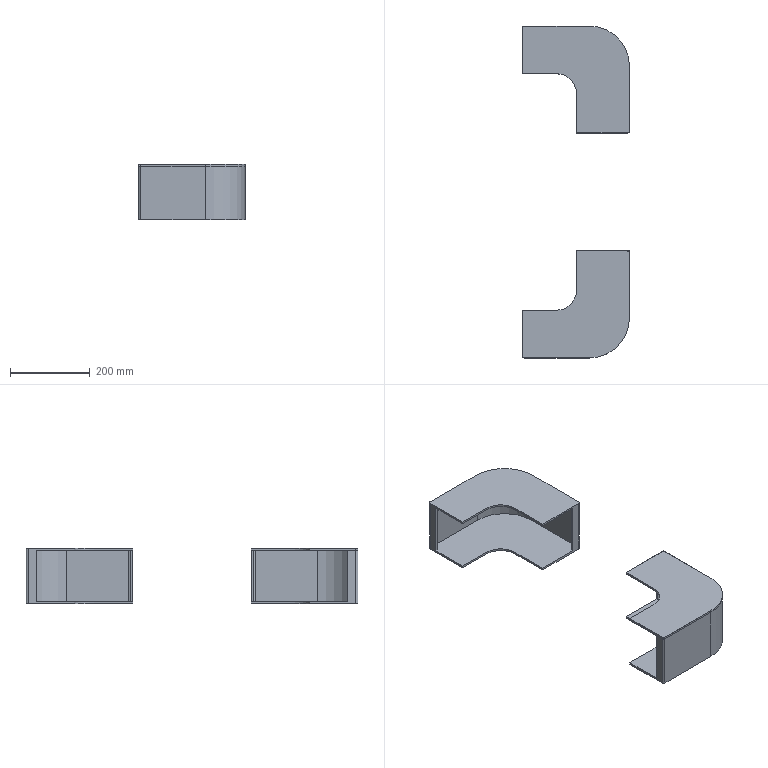Part | NX | features BREP 3 | 3 solids | 62 faces | box 267.373 x 830 x 140 mm | volume 1932570 mm3 | plane 44 | cylinder 18 | commonest cylinder face diameters 10 x8 100 x5 200 x3 190 x2